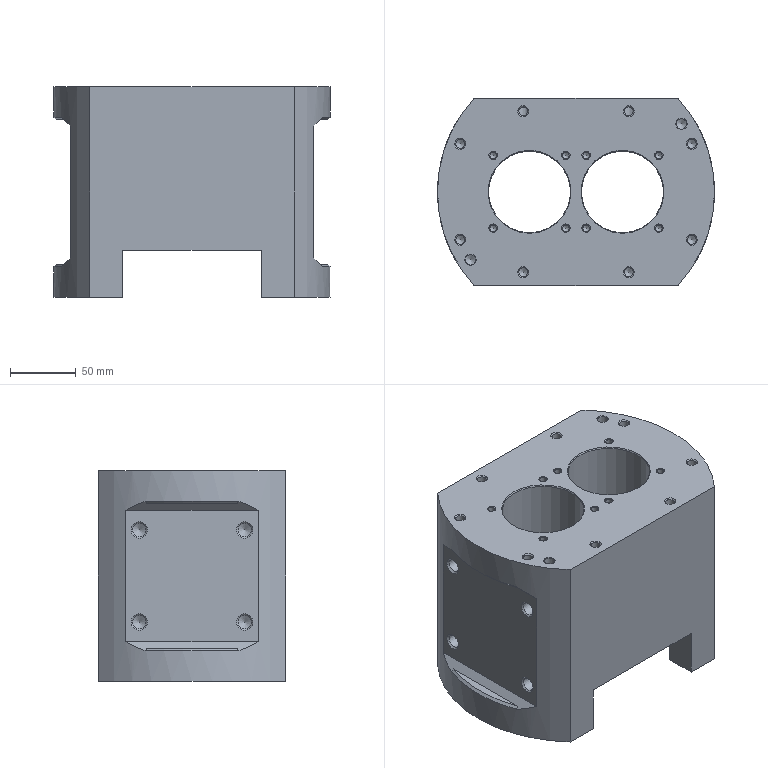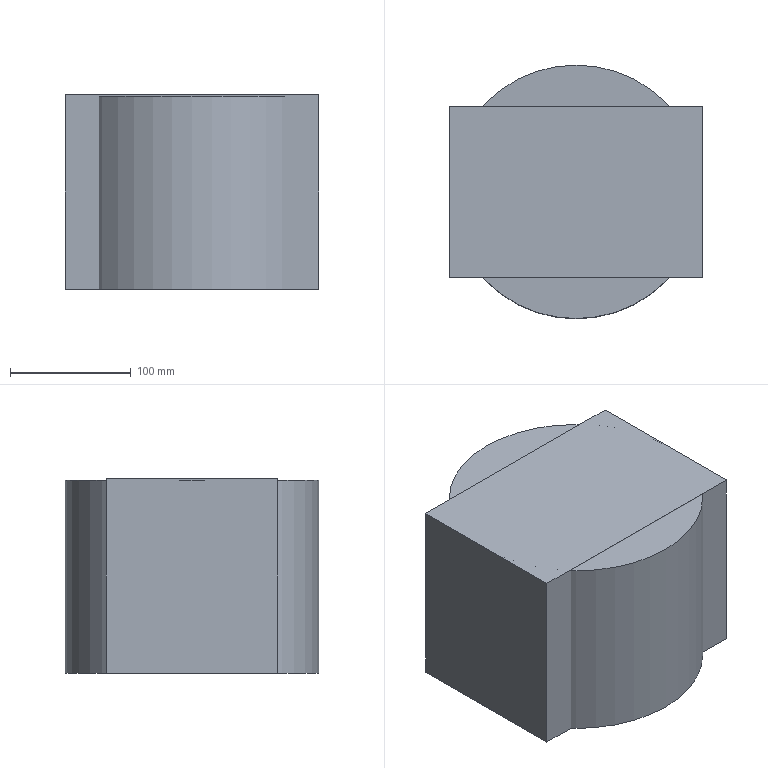CAM job | NX | 3+2 milling, drilling | part box 210 x 142 x 160 mm | stock box 210 x 210 x 161 mm
Tools:
number,name,description,diameter,corner_radius,flute_length,length,flutes
2,D50,Milling Tool-5 Parameters,50.0,0.0,50.0,75.0,2
1,ZXZ,Milling Tool-5 Parameters,6.0,0.0,50.0,75.0,2
11,10.2ZT,Drilling Tool,10.2,0.0,35.0,50.0,2
12,M12,Milling Tool-5 Parameters,10.2,0.0,30.0,30.0,4
7,D6A45,Milling Tool-5 Parameters,6.0,0.0,50.0,75.0,2
10,D10,Milling Tool-5 Parameters,10.0,0.0,50.0,75.0,2
5,D6R0.5,Milling Tool-5 Parameters,6.0,0.5,50.0,75.0,2
16,6.8ZT,Drilling Tool,6.8,0.0,35.0,50.0,2
18,M8,Milling Tool-5 Parameters,6.8,0.0,30.0,30.0,4
15,5.2ZT,Drilling Tool,5.0,0.0,35.0,50.0,2
14,M6,Milling Tool-5 Parameters,5.0,0.0,30.0,30.0,4
17,7.8ZT,Drilling Tool,7.8,0.0,35.0,50.0,2
18,8.0JD,Milling Tool-5 Parameters,8.0,0.0,30.0,30.0,4
19,11.8ZT,Drilling Tool,11.8,0.0,35.0,50.0,2
9,D35R.5,Milling Tool-5 Parameters,35.0,0.5,50.0,75.0,2
8,62.0JD,Milling Tool-5 Parameters,62.0,0.0,50.0,75.0,2
11,D10JING,Milling Tool-5 Parameters,10.0,0.0,50.0,75.0,2
20,8.5ZT,Drilling Tool,8.5,0.0,35.0,50.0,2
21,M10,Milling Tool-5 Parameters,8.5,0.0,30.0,30.0,4
3,9.8ZT,Drilling Tool,9.8,0.0,35.0,50.0,2
4,10.JD,Milling Tool-5 Parameters,10.0,0.0,30.0,30.0,4
Operations:
program,operation,operation_type,tool,method,geometry_group,spindle_rpm,surface_speed,feed_per_tooth,feed_cut,feed_plunge,cut_length_mm,path_length_mm,cut_time_min,machine_time_min
1,FLOOR_WALL,VolumeBased25DMillingOperation,D50,METHOD,A,1200.0,188.0,0.8333,2000.0,1000.0,102841.11,134911.332,51.712,54.919
1,FLOOR_WALL_COPY,VolumeBased25DMillingOperation,D50,METHOD,A,2500.0,392.0,0.2,1000.0,1000.0,1295.56,1417.56,1.296,1.308
1,DRILLING,Operation,ZXZ,METHOD,A,5000.0,94.0,0.025,250.0,0.0,16.0,389.185,0.064,0.1013
1,DRILLING_COPY,Operation,10.2ZT,METHOD,A,1200.0,38.0,0.1042,250.0,0.0,128.258,639.987,0.513,0.5642
1,DRILLING_COPY_COPY,Operation,M12,METHOD,A,200.0,6.0,0.0022,1.75,0.0,116.0,615.472,66.286,66.336
1,PLANAR_MILL_COPY_COPY,PlanarMilling,D6A45,METHOD,A,7500.0,141.0,0.0833,1250.0,100.0,165.459,899.593,0.1324,0.2058
2,FLOOR_WALL_COPY_1,VolumeBased25DMillingOperation,D50,METHOD,B,1200.0,188.0,0.8333,2000.0,1000.0,102841.11,134911.331,51.712,54.919
2,FLOOR_WALL_COPY_COPY,VolumeBased25DMillingOperation,D50,METHOD,B,2500.0,392.0,0.2,1000.0,1000.0,1295.56,1417.56,1.296,1.308
3,FLOOR_WALL_COPY_1_COPY,VolumeBased25DMillingOperation,D50,METHOD,C,1200.0,188.0,0.8333,2000.0,1000.0,15479.811,22818.151,7.851,8.585
3,FLOOR_WALL_COPY_COPY_COPY,VolumeBased25DMillingOperation,D50,METHOD,C,2500.0,392.0,0.2,1000.0,1000.0,512.892,592.392,0.5129,0.5208
3,ZLEVEL_PROFILE_COPY,ZLevelMilling,D10,METHOD,C,3500.0,109.0,0.3143,2200.0,1000.0,16891.12,17159.958,7.684,7.711
3,ZLEVEL_PROFILE,ZLevelMilling,D6R0.5,METHOD,C,6500.0,122.0,0.1923,2500.0,1000.0,26364.054,26616.918,10.551,10.576
3,DRILLING_COPY_1,Operation,ZXZ,METHOD,C,5000.0,94.0,0.025,250.0,0.0,16.0,346.685,0.064,0.0971
3,DRILLING_COPY_COPY_1,Operation,10.2ZT,METHOD,C,1200.0,38.0,0.1042,250.0,0.0,128.258,571.2,0.513,0.5573
3,DRILLING_COPY_COPY_COPY,Operation,M12,METHOD,C,200.0,6.0,0.0022,1.75,0.0,116.0,546.685,66.286,66.329
3,PLANAR_MILL_COPY_COPY_COPY,PlanarMilling,D6A45,METHOD,C,7500.0,141.0,0.0833,1250.0,100.0,165.459,729.269,0.1324,0.1887
4,FLOOR_WALL_COPY_1_COPY_COPY,VolumeBased25DMillingOperation,D50,METHOD,D,1200.0,188.0,0.8333,2000.0,1000.0,15479.811,22818.151,7.851,8.585
4,FLOOR_WALL_COPY_COPY_COPY_COPY,VolumeBased25DMillingOperation,D50,METHOD,D,2500.0,392.0,0.2,1000.0,1000.0,512.892,592.392,0.5129,0.5208
4,ZLEVEL_PROFILE_COPY_COPY,ZLevelMilling,D10,METHOD,D,3500.0,109.0,0.3143,2200.0,1000.0,16891.352,17160.191,7.684,7.711
4,ZLEVEL_PROFILE_COPY_1,ZLevelMilling,D6R0.5,METHOD,D,6500.0,122.0,0.1923,2500.0,1000.0,26366.589,26619.453,10.552,10.578
5,FLOOR_WALL_COPY_COPY_COPY_COPY_1,VolumeBased25DMillingOperation,D50,METHOD,E,2500.0,392.0,0.2,1000.0,1000.0,1393.064,1446.065,1.393,1.398
5,DRILLING_COPY_2,Operation,ZXZ,METHOD,E,5000.0,94.0,0.025,250.0,0.0,80.0,922.393,0.32,0.4042
5,DRILLING_COPY_2_COPY,Operation,6.8ZT,METHOD,E,2000.0,42.0,0.05,200.0,0.0,235.741,993.422,1.179,1.254
5,DRILLING_COPY_2_COPY_COPY,Operation,M8,METHOD,E,200.0,4.0,0.0016,1.25,0.0,219.397,960.735,175.518,175.592
5,DRILLING_COPY_2_COPY_COPY_1,Operation,5.2ZT,METHOD,E,2000.0,42.0,0.05,200.0,0.0,196.017,780.486,0.9801,1.038
5,DRILLING_COPY_2_COPY_COPY_1_COPY,Operation,M6,METHOD,E,200.0,3.0,0.0013,1.0,0.0,184.0,756.452,184.0,184.057
5,DRILLING_COPY_2_COPY_COPY_1_COPY_1,Operation,7.8ZT,METHOD,E,2000.0,42.0,0.05,200.0,0.0,50.807,354.924,0.254,0.2844
5,DRILLING_COPY_2_COPY_COPY_1_COPY_1_COPY,Operation,8.0JD,METHOD,E,1000.0,25.0,0.01,40.0,0.0,46.0,345.31,1.15,1.18
5,DRILLING_COPY_COPY_1_COPY,Operation,11.8ZT,METHOD,E,1025.0,38.0,0.0732,150.0,0.0,264.09,661.744,1.761,1.8
5,HOLE_MILLING,CylinderMilling,D35R.5,METHOD,E,1500.0,164.0,0.4,1200.0,100.0,85474.632,85915.132,71.229,71.273
5,DRILLING_COPY_2_COPY_COPY_1_COPY_1_COPY_COPY,Operation,62.0JD,METHOD,E,300.0,64.0,0.0667,40.0,0.0,255.0,643.564,6.375,6.414
5,PLANAR_MILL_COPY_COPY_COPY_COPY,PlanarMilling,D6A45,METHOD,E,7500.0,141.0,0.0833,1250.0,100.0,832.715,2593.973,0.6662,0.8423
5,PLANAR_MILL_COPY_COPY_COPY_COPY_COPY,PlanarMilling,D6A45,METHOD,E,7500.0,141.0,0.0833,1250.0,100.0,639.382,696.382,0.5115,0.5172
6,FLOOR_WALL_COPY_COPY_COPY_COPY_1_COPY,VolumeBased25DMillingOperation,D50,METHOD,F,2500.0,392.0,0.2,1000.0,1000.0,1433.997,1487.997,1.434,1.439
6,FLOOR_WALL_1,VolumeBased25DMillingOperation,D50,METHOD,F,1200.0,188.0,0.8333,2000.0,1000.0,75542.879,83479.577,39.398,40.191
6,FLOOR_WALL_2_COPY,VolumeBased25DMillingOperation,D10JING,METHOD,F,5000.0,157.0,0.12,1200.0,500.0,3117.527,6054.527,2.71,3.004
6,FLOOR_WALL_2,VolumeBased25DMillingOperation,D10JING,METHOD,F,5000.0,157.0,0.12,1200.0,500.0,4542.732,5098.399,3.756,3.812
6,DRILLING_COPY_2_COPY_1,Operation,ZXZ,METHOD,F,5000.0,94.0,0.025,250.0,0.0,64.0,892.295,0.256,0.3388
6,DRILLING_COPY_2_COPY_COPY_1_COPY_2,Operation,5.2ZT,METHOD,F,2000.0,42.0,0.05,200.0,0.0,196.017,852.486,0.9801,1.046
6,DRILLING_COPY_2_COPY_COPY_1_COPY_COPY,Operation,M6,METHOD,F,200.0,3.0,0.0013,1.0,0.0,184.0,828.452,184.0,184.064
6,DRILLING_COPY_2_COPY_COPY_1_COPY_2_COPY,Operation,8.5ZT,METHOD,F,2000.0,53.0,0.05,200.0,0.0,140.215,723.538,0.7011,0.7594
6,DRILLING_COPY_2_COPY_COPY_1_COPY_2_COPY_COPY,Operation,M10,METHOD,F,200.0,5.0,0.0019,1.5,0.0,130.0,703.109,86.667,86.724
6,DRILLING_COPY_2_COPY_COPY_1_COPY_1_COPY_1,Operation,9.8ZT,METHOD,F,2000.0,42.0,0.05,200.0,0.0,52.009,356.07,0.26,0.2904
6,DRILLING_COPY_2_COPY_COPY_1_COPY_1_COPY_COPY_1,Operation,10.JD,METHOD,F,1000.0,25.0,0.01,40.0,0.0,46.0,344.053,1.15,1.18
6,PLANAR_MILL_COPY_COPY_COPY_COPY_COPY_1,PlanarMilling,D6A45,METHOD,F,7500.0,141.0,0.0833,1250.0,100.0,198.982,936.591,0.1592,0.2329
6,PLANAR_MILL_COPY_COPY_COPY_COPY_COPY_1_COPY,PlanarMilling,D6A45,METHOD,F,7500.0,141.0,0.0833,1250.0,100.0,563.225,2231.761,0.4506,0.6174
6,PLANAR_MILL_COPY_COPY_COPY_COPY_COPY_COPY,PlanarMilling,D6A45,METHOD,F,7500.0,141.0,0.0833,1250.0,100.0,789.086,1036.001,0.6313,0.656
6,PLANAR_MILL_COPY_COPY_COPY_COPY_COPY_COPY_COPY,PlanarMilling,D6A45,METHOD,F,7500.0,141.0,0.0833,1250.0,100.0,215.912,621.707,0.1727,0.2133